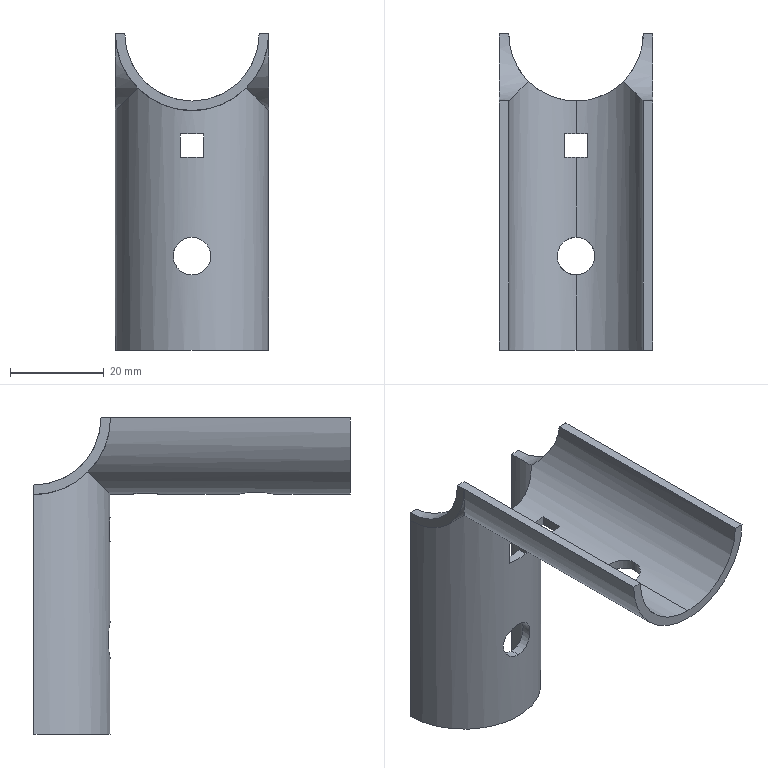Part | STEP file | F-A | 1 solid | 30 faces | box 32.6 x 67.3 x 67.3 mm | volume 10224 mm3 | plane 16 | cylinder 14 | commonest cylinder face diameters 28.6 x5 32.6 x5 8 x4